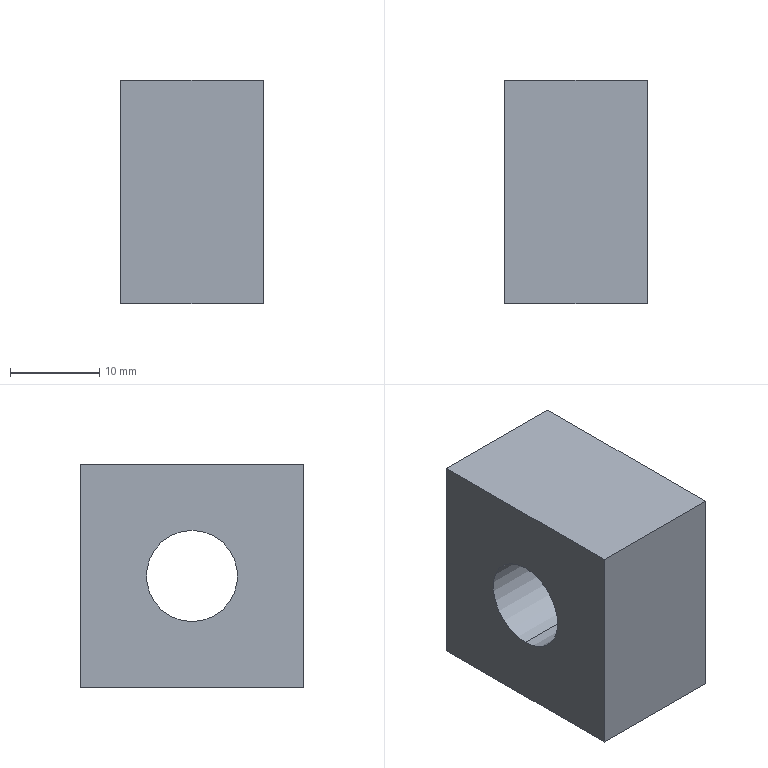Part | SolidWorks | features FlatPattern 1, HoleWzd 1, SMBaseFlange 1, SheetMetal 1 | 1 solid | 8 faces | box 16 x 25 x 25 mm | volume 8693 mm3 | plane 6 | cylinder 2 | commonest cylinder face diameters 10.2 x2
STEP:
#1=CARTESIAN_POINT('',(-16.,0.,5.1));
#2=VERTEX_POINT('',#1);
#3=CARTESIAN_POINT('',(-16.,0.,-5.1));
#4=VERTEX_POINT('',#3);
#5=CARTESIAN_POINT('',(-16.,0.,0.));
#6=DIRECTION('',(1.,0.,0.));
#7=DIRECTION('',(0.,0.,-1.));
#8=AXIS2_PLACEMENT_3D('',#5,#6,#7);
#9=CIRCLE('',#8,5.1);
#10=EDGE_CURVE('',#2,#4,#9,.T.);
#11=ORIENTED_EDGE('',*,*,#10,.F.);
#12=CARTESIAN_POINT('',(0.,0.,5.1));
#13=VERTEX_POINT('',#12);
#14=CARTESIAN_POINT('',(0.,0.,5.1));
#15=DIRECTION('',(1.,0.,0.));
#16=VECTOR('',#15,1000.);
#17=LINE('',#14,#16);
#18=EDGE_CURVE('',#2,#13,#17,.T.);
#19=ORIENTED_EDGE('',*,*,#18,.T.);
#20=CARTESIAN_POINT('',(0.,0.,-5.1));
#21=VERTEX_POINT('',#20);
#22=CARTESIAN_POINT('',(0.,0.,0.));
#23=DIRECTION('',(1.,0.,0.));
#24=DIRECTION('',(0.,0.,-1.));
#25=AXIS2_PLACEMENT_3D('',#22,#23,#24);
#26=CIRCLE('',#25,5.1);
#27=EDGE_CURVE('',#13,#21,#26,.T.);
#28=ORIENTED_EDGE('',*,*,#27,.T.);
#29=CARTESIAN_POINT('',(0.,0.,-5.1));
#30=DIRECTION('',(1.,0.,0.));
#31=VECTOR('',#30,1000.);
#32=LINE('',#29,#31);
#33=EDGE_CURVE('',#4,#21,#32,.T.);
#34=ORIENTED_EDGE('',*,*,#33,.F.);
#35=EDGE_LOOP('',(#11,#19,#28,#34));
#36=FACE_OUTER_BOUND('',#35,.T.);
#37=CARTESIAN_POINT('',(0.,0.,0.));
#38=DIRECTION('',(1.,0.,0.));
#39=DIRECTION('',(0.,0.,-1.));
#40=AXIS2_PLACEMENT_3D('',#37,#38,#39);
#41=CYLINDRICAL_SURFACE('',#40,5.1);
#42=ADVANCED_FACE('',(#36),#41,.F.);
#43=CARTESIAN_POINT('',(0.,-12.5,-12.5));
#44=VERTEX_POINT('',#43);
#45=CARTESIAN_POINT('',(0.,12.5,-12.5));
#46=VERTEX_POINT('',#45);
#47=CARTESIAN_POINT('',(0.,12.5,-12.5));
#48=DIRECTION('',(0.,1.,0.));
#49=VECTOR('',#48,1000.);
#50=LINE('',#47,#49);
#51=EDGE_CURVE('',#44,#46,#50,.T.);
#52=ORIENTED_EDGE('',*,*,#51,.F.);
#53=CARTESIAN_POINT('',(-16.,-12.5,-12.5));
#54=VERTEX_POINT('',#53);
#55=CARTESIAN_POINT('',(-16.,-12.5,-12.5));
#56=DIRECTION('',(1.,0.,0.));
#57=VECTOR('',#56,1000.);
#58=LINE('',#55,#57);
#59=EDGE_CURVE('',#54,#44,#58,.T.);
#60=ORIENTED_EDGE('',*,*,#59,.F.);
#61=CARTESIAN_POINT('',(-16.,12.5,-12.5));
#62=VERTEX_POINT('',#61);
#63=CARTESIAN_POINT('',(-16.,12.5,-12.5));
#64=DIRECTION('',(0.,1.,0.));
#65=VECTOR('',#64,1000.);
#66=LINE('',#63,#65);
#67=EDGE_CURVE('',#54,#62,#66,.T.);
#68=ORIENTED_EDGE('',*,*,#67,.T.);
#69=CARTESIAN_POINT('',(-16.,12.5,-12.5));
#70=DIRECTION('',(1.,0.,0.));
#71=VECTOR('',#70,1000.);
#72=LINE('',#69,#71);
#73=EDGE_CURVE('',#62,#46,#72,.T.);
#74=ORIENTED_EDGE('',*,*,#73,.T.);
#75=EDGE_LOOP('',(#52,#60,#68,#74));
#76=FACE_OUTER_BOUND('',#75,.T.);
#77=CARTESIAN_POINT('',(-16.,12.5,-12.5));
#78=DIRECTION('',(0.,0.,-1.));
#79=DIRECTION('',(0.,1.,0.));
#80=AXIS2_PLACEMENT_3D('',#77,#78,#79);
#81=PLANE('',#80);
#82=ADVANCED_FACE('',(#76),#81,.T.);
#83=CARTESIAN_POINT('',(0.,-12.5,12.5));
#84=VERTEX_POINT('',#83);
#85=CARTESIAN_POINT('',(0.,-12.5,12.5));
#86=DIRECTION('',(0.,0.,-1.));
#87=VECTOR('',#86,1000.);
#88=LINE('',#85,#87);
#89=EDGE_CURVE('',#84,#44,#88,.T.);
#90=ORIENTED_EDGE('',*,*,#89,.F.);
#91=CARTESIAN_POINT('',(-16.,-12.5,12.5));
#92=VERTEX_POINT('',#91);
#93=CARTESIAN_POINT('',(-16.,-12.5,12.5));
#94=DIRECTION('',(1.,0.,0.));
#95=VECTOR('',#94,1000.);
#96=LINE('',#93,#95);
#97=EDGE_CURVE('',#92,#84,#96,.T.);
#98=ORIENTED_EDGE('',*,*,#97,.F.);
#99=CARTESIAN_POINT('',(-16.,-12.5,12.5));
#100=DIRECTION('',(0.,0.,-1.));
#101=VECTOR('',#100,1000.);
#102=LINE('',#99,#101);
#103=EDGE_CURVE('',#92,#54,#102,.T.);
#104=ORIENTED_EDGE('',*,*,#103,.T.);
#105=ORIENTED_EDGE('',*,*,#59,.T.);
#106=EDGE_LOOP('',(#90,#98,#104,#105));
#107=FACE_OUTER_BOUND('',#106,.T.);
#108=CARTESIAN_POINT('',(-16.,-12.5,12.5));
#109=DIRECTION('',(0.,-1.,0.));
#110=DIRECTION('',(0.,0.,-1.));
#111=AXIS2_PLACEMENT_3D('',#108,#109,#110);
#112=PLANE('',#111);
#113=ADVANCED_FACE('',(#107),#112,.T.);
#114=CARTESIAN_POINT('',(0.,12.5,12.5));
#115=VERTEX_POINT('',#114);
#116=CARTESIAN_POINT('',(0.,12.5,12.5));
#117=DIRECTION('',(0.,-1.,0.));
#118=VECTOR('',#117,1000.);
#119=LINE('',#116,#118);
#120=EDGE_CURVE('',#115,#84,#119,.T.);
#121=ORIENTED_EDGE('',*,*,#120,.F.);
#122=CARTESIAN_POINT('',(-16.,12.5,12.5));
#123=VERTEX_POINT('',#122);
#124=CARTESIAN_POINT('',(-16.,12.5,12.5));
#125=DIRECTION('',(1.,0.,0.));
#126=VECTOR('',#125,1000.);
#127=LINE('',#124,#126);
#128=EDGE_CURVE('',#123,#115,#127,.T.);
#129=ORIENTED_EDGE('',*,*,#128,.F.);
#130=CARTESIAN_POINT('',(-16.,12.5,12.5));
#131=DIRECTION('',(0.,-1.,0.));
#132=VECTOR('',#131,1000.);
#133=LINE('',#130,#132);
#134=EDGE_CURVE('',#123,#92,#133,.T.);
#135=ORIENTED_EDGE('',*,*,#134,.T.);
#136=ORIENTED_EDGE('',*,*,#97,.T.);
#137=EDGE_LOOP('',(#121,#129,#135,#136));
#138=FACE_OUTER_BOUND('',#137,.T.);
#139=CARTESIAN_POINT('',(-16.,12.5,12.5));
#140=DIRECTION('',(0.,0.,1.));
#141=DIRECTION('',(0.,-1.,0.));
#142=AXIS2_PLACEMENT_3D('',#139,#140,#141);
#143=PLANE('',#142);
#144=ADVANCED_FACE('',(#138),#143,.T.);
#145=CARTESIAN_POINT('',(0.,12.5,12.5));
#146=DIRECTION('',(0.,0.,1.));
#147=VECTOR('',#146,1000.);
#148=LINE('',#145,#147);
#149=EDGE_CURVE('',#46,#115,#148,.T.);
#150=ORIENTED_EDGE('',*,*,#149,.F.);
#151=ORIENTED_EDGE('',*,*,#73,.F.);
#152=CARTESIAN_POINT('',(-16.,12.5,12.5));
#153=DIRECTION('',(0.,0.,1.));
#154=VECTOR('',#153,1000.);
#155=LINE('',#152,#154);
#156=EDGE_CURVE('',#62,#123,#155,.T.);
#157=ORIENTED_EDGE('',*,*,#156,.T.);
#158=ORIENTED_EDGE('',*,*,#128,.T.);
#159=EDGE_LOOP('',(#150,#151,#157,#158));
#160=FACE_OUTER_BOUND('',#159,.T.);
#161=CARTESIAN_POINT('',(-16.,12.5,12.5));
#162=DIRECTION('',(0.,1.,0.));
#163=DIRECTION('',(0.,0.,1.));
#164=AXIS2_PLACEMENT_3D('',#161,#162,#163);
#165=PLANE('',#164);
#166=ADVANCED_FACE('',(#160),#165,.T.);
#167=CARTESIAN_POINT('',(-16.,0.,0.));
#168=DIRECTION('',(1.,0.,0.));
#169=DIRECTION('',(0.,0.,-1.));
#170=AXIS2_PLACEMENT_3D('',#167,#168,#169);
#171=CIRCLE('',#170,5.1);
#172=EDGE_CURVE('',#4,#2,#171,.T.);
#173=ORIENTED_EDGE('',*,*,#172,.T.);
#174=ORIENTED_EDGE('',*,*,#10,.T.);
#175=EDGE_LOOP('',(#173,#174));
#176=FACE_BOUND('',#175,.T.);
#177=ORIENTED_EDGE('',*,*,#67,.F.);
#178=ORIENTED_EDGE('',*,*,#103,.F.);
#179=ORIENTED_EDGE('',*,*,#134,.F.);
#180=ORIENTED_EDGE('',*,*,#156,.F.);
#181=EDGE_LOOP('',(#177,#178,#179,#180));
#182=FACE_OUTER_BOUND('',#181,.T.);
#183=CARTESIAN_POINT('',(-16.,0.,0.));
#184=DIRECTION('',(1.,0.,0.));
#185=DIRECTION('',(0.,0.,-1.));
#186=AXIS2_PLACEMENT_3D('',#183,#184,#185);
#187=PLANE('',#186);
#188=ADVANCED_FACE('',(#176,#182),#187,.F.);
#189=CARTESIAN_POINT('',(0.,0.,0.));
#190=DIRECTION('',(1.,0.,0.));
#191=DIRECTION('',(0.,0.,-1.));
#192=AXIS2_PLACEMENT_3D('',#189,#190,#191);
#193=CIRCLE('',#192,5.1);
#194=EDGE_CURVE('',#21,#13,#193,.T.);
#195=ORIENTED_EDGE('',*,*,#194,.F.);
#196=ORIENTED_EDGE('',*,*,#27,.F.);
#197=EDGE_LOOP('',(#195,#196));
#198=FACE_BOUND('',#197,.T.);
#199=ORIENTED_EDGE('',*,*,#51,.T.);
#200=ORIENTED_EDGE('',*,*,#149,.T.);
#201=ORIENTED_EDGE('',*,*,#120,.T.);
#202=ORIENTED_EDGE('',*,*,#89,.T.);
#203=EDGE_LOOP('',(#199,#200,#201,#202));
#204=FACE_OUTER_BOUND('',#203,.T.);
#205=CARTESIAN_POINT('',(0.,0.,0.));
#206=DIRECTION('',(1.,0.,0.));
#207=DIRECTION('',(0.,0.,-1.));
#208=AXIS2_PLACEMENT_3D('',#205,#206,#207);
#209=PLANE('',#208);
#210=ADVANCED_FACE('',(#198,#204),#209,.T.);
#211=ORIENTED_EDGE('',*,*,#18,.F.);
#212=ORIENTED_EDGE('',*,*,#172,.F.);
#213=ORIENTED_EDGE('',*,*,#33,.T.);
#214=ORIENTED_EDGE('',*,*,#194,.T.);
#215=EDGE_LOOP('',(#211,#212,#213,#214));
#216=FACE_OUTER_BOUND('',#215,.T.);
#217=CARTESIAN_POINT('',(0.,0.,0.));
#218=DIRECTION('',(1.,0.,0.));
#219=DIRECTION('',(0.,0.,-1.));
#220=AXIS2_PLACEMENT_3D('',#217,#218,#219);
#221=CYLINDRICAL_SURFACE('',#220,5.1);
#222=ADVANCED_FACE('',(#216),#221,.F.);
#223=CLOSED_SHELL('',(#42,#82,#113,#144,#166,#188,#210,#222));
#224=MANIFOLD_SOLID_BREP('',#223);
#225=CARTESIAN_POINT('',(0.,0.,0.));
#226=DIRECTION('',(0.,0.,1.));
#227=DIRECTION('',(1.,0.,0.));
#228=AXIS2_PLACEMENT_3D('',#225,#226,#227);
#229=(LENGTH_UNIT()NAMED_UNIT(*)SI_UNIT(.MILLI.,.METRE.));
#230=UNCERTAINTY_MEASURE_WITH_UNIT(LENGTH_MEASURE(0.00001),#229,'','');
#231=(NAMED_UNIT(*)PLANE_ANGLE_UNIT()SI_UNIT($,.RADIAN.));
#232=(NAMED_UNIT(*)SI_UNIT($,.STERADIAN.)SOLID_ANGLE_UNIT());
#233=(GEOMETRIC_REPRESENTATION_CONTEXT(3)GLOBAL_UNCERTAINTY_ASSIGNED_CONTEXT((#230))GLOBAL_UNIT_ASSIGNED_CONTEXT((#229,#231,#232))REPRESENTATION_CONTEXT('',''));
#234=ADVANCED_BREP_SHAPE_REPRESENTATION('',(#224,#228),#233);